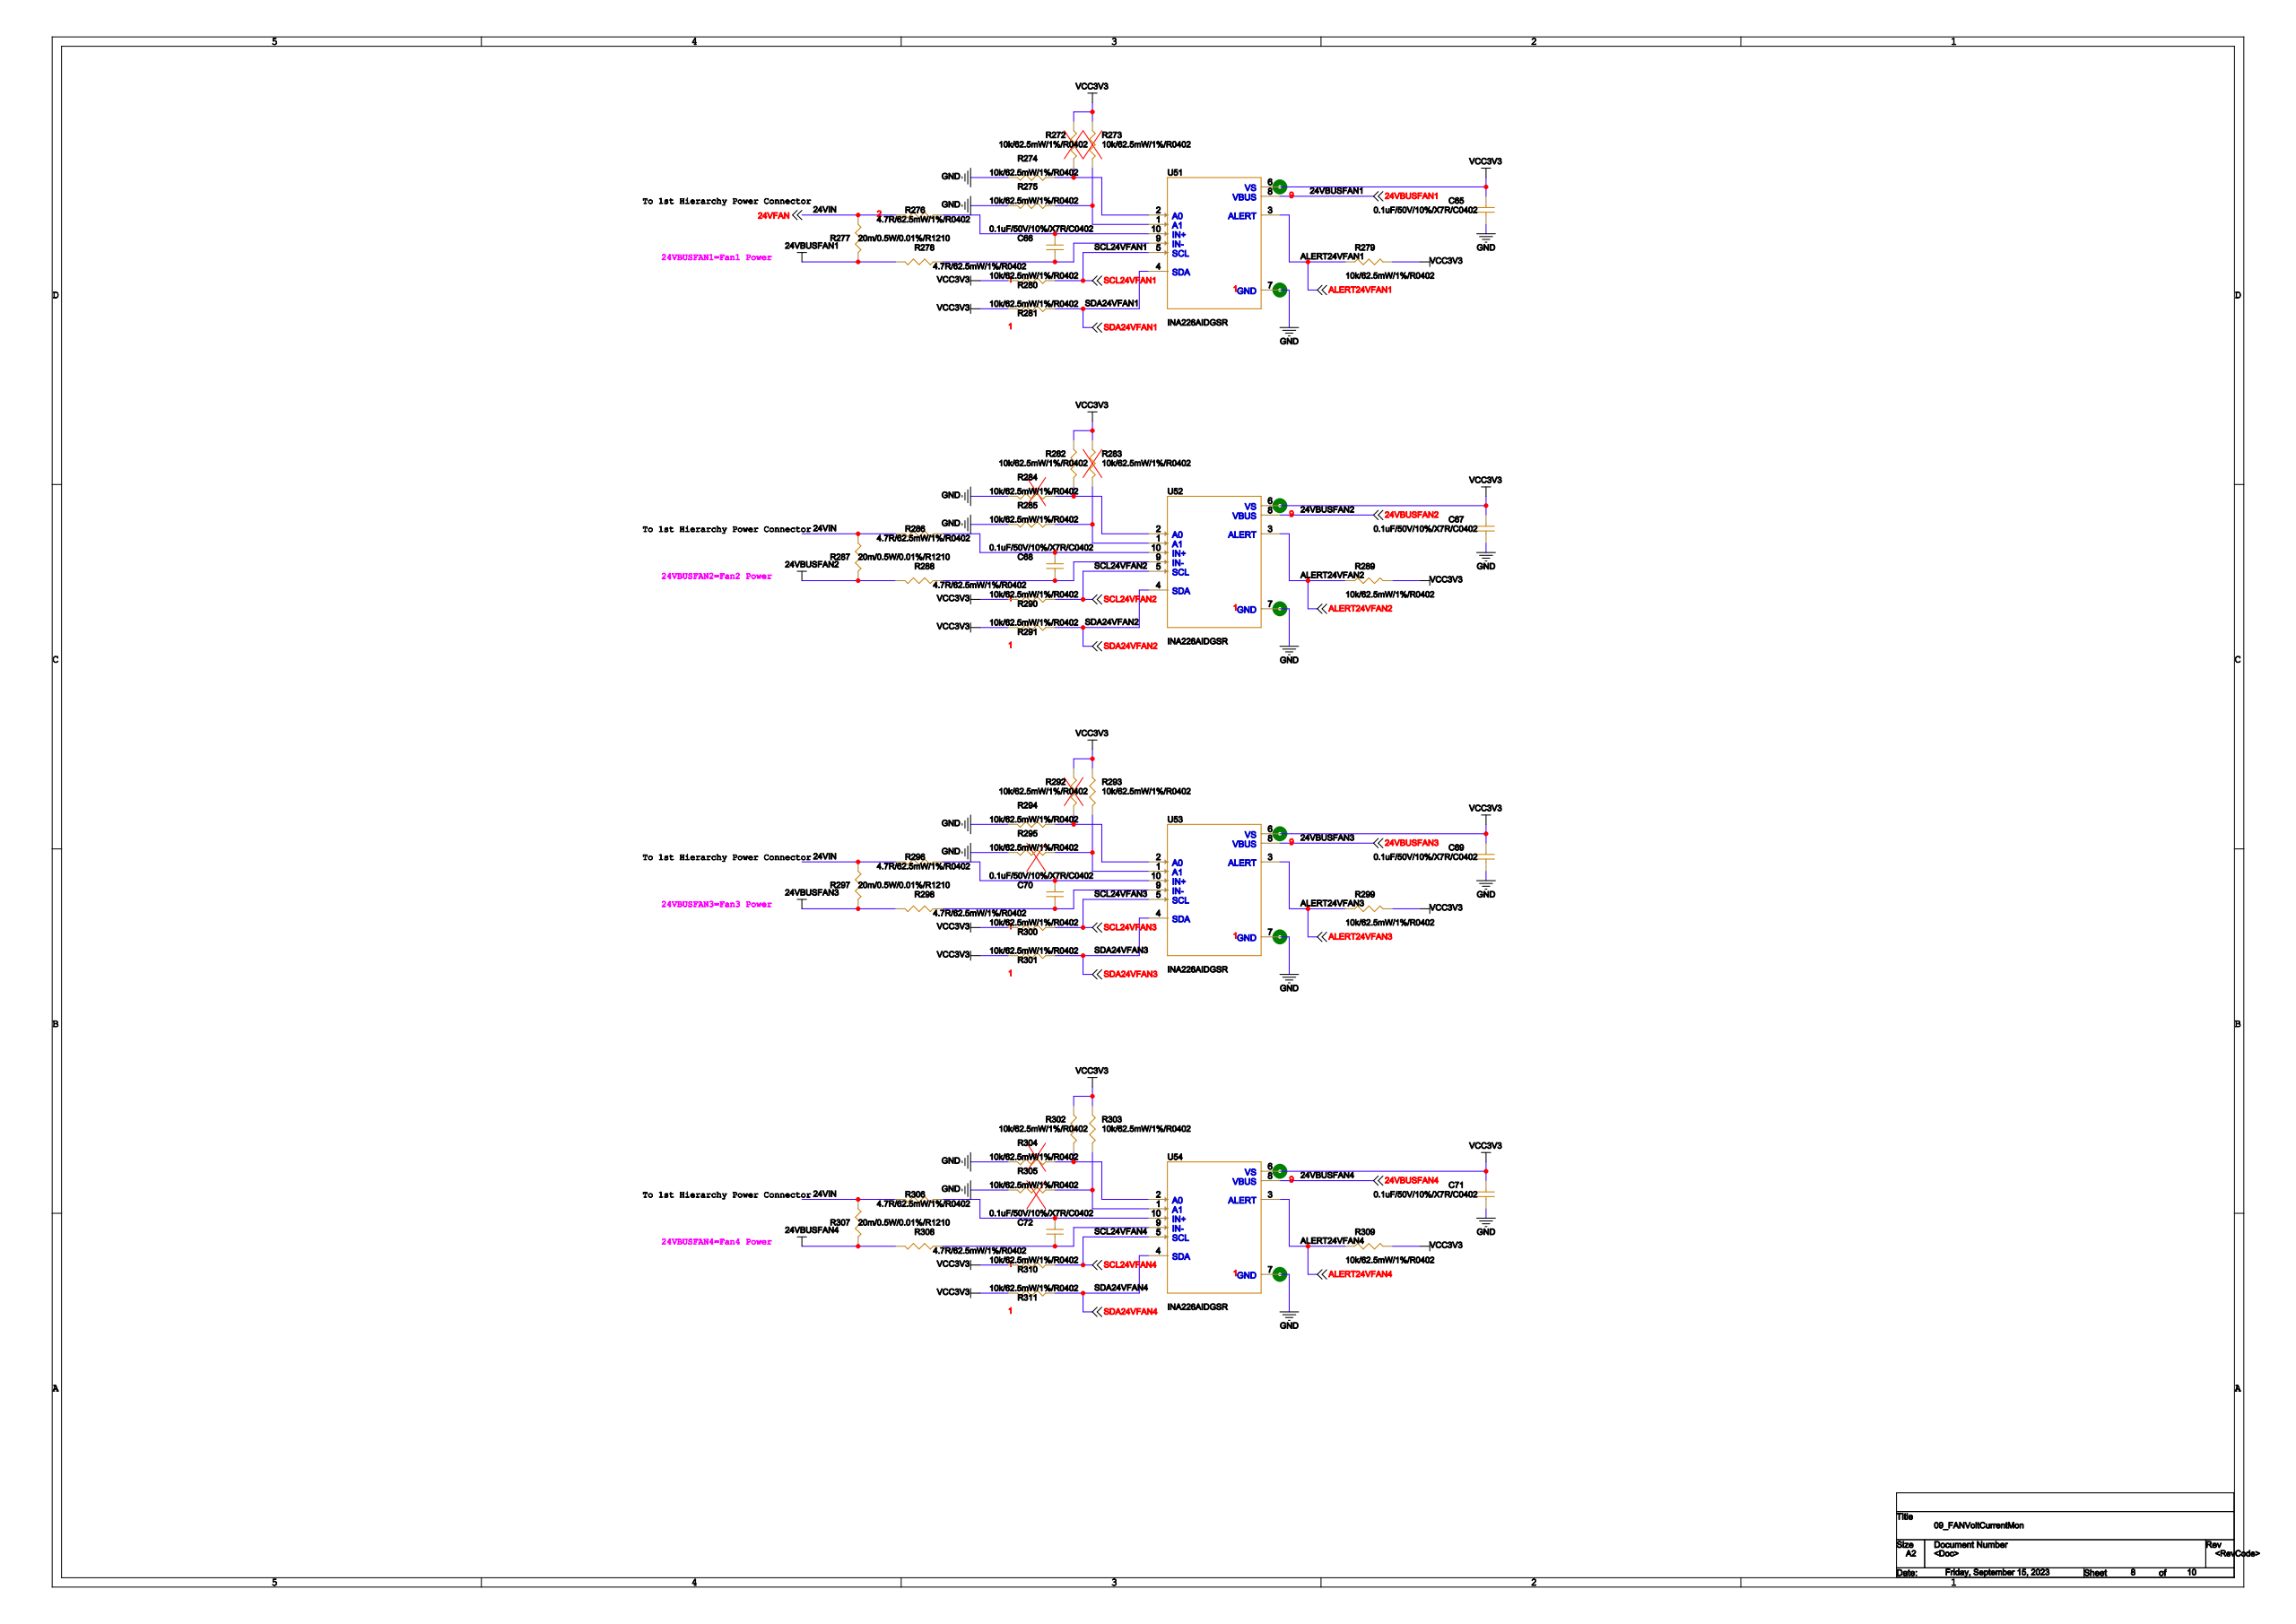Circuit board | Cadence Allegro | 634 parts | 645 nets | one sheet of the schematic
Parts on this sheet (reference | value | footprint):
C65 | 0.1uF/50V/10%/X7R/C0402 | 0402
C66 | 0.1uF/50V/10%/X7R/C0402 | 0402
C67 | 0.1uF/50V/10%/X7R/C0402 | 0402
C68 | 0.1uF/50V/10%/X7R/C0402 | 0402
C69 | 0.1uF/50V/10%/X7R/C0402 | 0402
C70 | 0.1uF/50V/10%/X7R/C0402 | 0402
C71 | 0.1uF/50V/10%/X7R/C0402 | 0402
C72 | 0.1uF/50V/10%/X7R/C0402 | 0402
R272 | 10k/62.5mW/1%/R0402 | 0402
R273 | 10k/62.5mW/1%/R0402 | 0402
R274 | 10k/62.5mW/1%/R0402 | 0402
R275 | 10k/62.5mW/1%/R0402 | 0402
R276 | 4.7R/62.5mW/1%/R0402 | 0402
R277 | 20m/0.5W/0.01%/R1210 | 1210
R278 | 4.7R/62.5mW/1%/R0402 | 0402
R279 | 10k/62.5mW/1%/R0402 | 0402
R280 | 10k/62.5mW/1%/R0402 | 0402
R281 | 10k/62.5mW/1%/R0402 | 0402
R282 | 10k/62.5mW/1%/R0402 | 0402
R283 | 10k/62.5mW/1%/R0402 | 0402
R284 | 10k/62.5mW/1%/R0402 | 0402
R285 | 10k/62.5mW/1%/R0402 | 0402
R286 | 4.7R/62.5mW/1%/R0402 | 0402
R287 | 20m/0.5W/0.01%/R1210 | 1210
R288 | 4.7R/62.5mW/1%/R0402 | 0402
R289 | 10k/62.5mW/1%/R0402 | 0402
R290 | 10k/62.5mW/1%/R0402 | 0402
R291 | 10k/62.5mW/1%/R0402 | 0402
R292 | 10k/62.5mW/1%/R0402 | 0402
R293 | 10k/62.5mW/1%/R0402 | 0402
R294 | 10k/62.5mW/1%/R0402 | 0402
R295 | 10k/62.5mW/1%/R0402 | 0402
R296 | 4.7R/62.5mW/1%/R0402 | 0402
R297 | 20m/0.5W/0.01%/R1210 | 1210
R298 | 4.7R/62.5mW/1%/R0402 | 0402
R299 | 10k/62.5mW/1%/R0402 | 0402
R300 | 10k/62.5mW/1%/R0402 | 0402
R301 | 10k/62.5mW/1%/R0402 | 0402
R302 | 10k/62.5mW/1%/R0402 | 0402
R303 | 10k/62.5mW/1%/R0402 | 0402
R304 | 10k/62.5mW/1%/R0402 | 0402
R305 | 10k/62.5mW/1%/R0402 | 0402
R306 | 4.7R/62.5mW/1%/R0402 | 0402
R307 | 20m/0.5W/0.01%/R1210 | 1210
R308 | 4.7R/62.5mW/1%/R0402 | 0402
R309 | 10k/62.5mW/1%/R0402 | 0402
R310 | 10k/62.5mW/1%/R0402 | 0402
R311 | 10k/62.5mW/1%/R0402 | 0402
U51 | INA226AIDGSR | SOP50P490X110-10N
U52 | INA226AIDGSR | SOP50P490X110-10N
U53 | INA226AIDGSR | SOP50P490X110-10N
U54 | INA226AIDGSR | SOP50P490X110-10N
Nets of these parts (net: part-pin ...):
AGND: C65-2 C67-2 C69-2 C71-2 R274-2 R275-2 R284-2 R285-2 R294-2 R295-2 R304-2 R305-2 U51-7 U52-7 U53-7 U54-7
SDA24VFAN3: R301-1 U53-4
SCL24VFAN3: R300-1 U53-5
ALERT24VFAN2: R289-1 U52-3
SDA24VFAN2: R291-1 U52-4
SCL24VFAN2: R290-1 U52-5
ALERT24VFAN1: R279-1 U51-3
SDA24VFAN1: R281-1 U51-4
SCL24VFAN1: R280-1 U51-5
3.3V: C65-1 C67-1 C69-1 C71-1 R272-1 R273-1 R279-2 R280-2 R281-2 R282-1 R283-1 R289-2 R290-2 R291-2 R292-1 R293-1 R299-2 R300-2 R301-2 R302-1 R303-1 R309-2 R310-2 R311-2 U51-6 U52-6 U53-6 U54-6
ALERT24VFAN4: R309-1 U54-3
SDA24VFAN4: R311-1 U54-4
SCL24VFAN4: R310-1 U54-5
ALERT24VFAN3: R299-1 U53-3
24VFAN: R276-2 R277-1 R286-2 R287-1 R296-2 R297-1 R306-2 R307-1
24VBUSFAN1: R277-2 R278-2 U51-8
24VBUSFAN2: R287-2 R288-2 U52-8
24VBUSFAN3: R297-2 R298-2 U53-8
24VBUSFAN4: R307-2 R308-2 U54-8
N23190079: C70-1 R296-1 U53-10
N23190245: C70-2 R298-1 U53-9
N23190745: C72-1 R306-1 U54-10
N23190911: C72-2 R308-1 U54-9
N23136700: C66-1 R276-1 U51-10
N23136726: C66-2 R278-1 U51-9
N23189446: C68-1 R286-1 U52-10
N23189612: C68-2 R288-1 U52-9
N23136475: R272-2 R274-1 U51-2
N23136485: R273-2 R275-1 U51-1
N23189541: R282-2 R284-1 U52-2
N23189547: R283-2 R285-1 U52-1
N23190174: R292-2 R294-1 U53-2
N23190180: R293-2 R295-1 U53-1
N23190840: R302-2 R304-1 U54-2
N23190846: R303-2 R305-1 U54-1